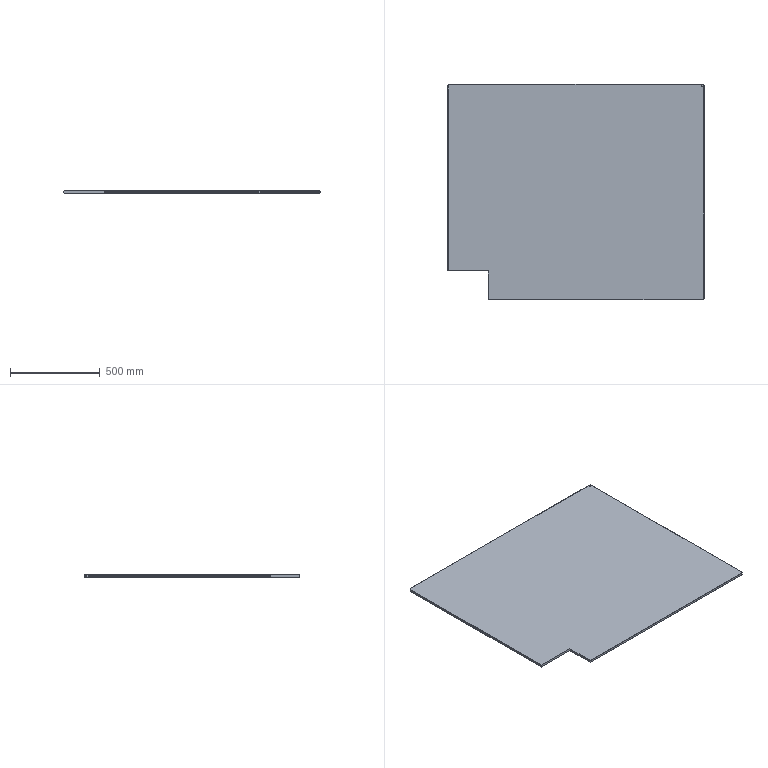Part | STEP file | 1200x1425x13 aluminium plateA-1.STEP | 1 solid | 27 faces | box 1425 x 1200 x 13 mm | volume 21754303 mm3 | plane 16 | cone 6 | cylinder 5 | commonest cylinder face diameters 20 x3 5 x2
STEP:
#1=CARTESIAN_POINT('',(-712.5,-439.4,1.));
#2=VERTEX_POINT('',#1);
#3=CARTESIAN_POINT('',(-711.5,-439.4,0.));
#4=VERTEX_POINT('',#3);
#5=CARTESIAN_POINT('',(-712.5,-439.4,1.));
#6=DIRECTION('',(0.7071,0.,-0.7071));
#7=VECTOR('',#6,1000.);
#8=LINE('',#5,#7);
#9=EDGE_CURVE('',#2,#4,#8,.T.);
#10=ORIENTED_EDGE('',*,*,#9,.T.);
#11=CARTESIAN_POINT('',(-487.5,-439.4,0.));
#12=VERTEX_POINT('',#11);
#13=CARTESIAN_POINT('',(-712.5,-439.4,0.));
#14=DIRECTION('',(1.,0.,0.));
#15=VECTOR('',#14,1000.);
#16=LINE('',#13,#15);
#17=EDGE_CURVE('',#4,#12,#16,.T.);
#18=ORIENTED_EDGE('',*,*,#17,.T.);
#19=CARTESIAN_POINT('',(-487.5,-439.4,13.));
#20=VERTEX_POINT('',#19);
#21=CARTESIAN_POINT('',(-487.5,-439.4,13.));
#22=DIRECTION('',(0.,0.,-1.));
#23=VECTOR('',#22,1000.);
#24=LINE('',#21,#23);
#25=EDGE_CURVE('',#20,#12,#24,.T.);
#26=ORIENTED_EDGE('',*,*,#25,.F.);
#27=CARTESIAN_POINT('',(-711.5,-439.4,13.));
#28=VERTEX_POINT('',#27);
#29=CARTESIAN_POINT('',(-712.5,-439.4,13.));
#30=DIRECTION('',(1.,0.,0.));
#31=VECTOR('',#30,1000.);
#32=LINE('',#29,#31);
#33=EDGE_CURVE('',#28,#20,#32,.T.);
#34=ORIENTED_EDGE('',*,*,#33,.F.);
#35=CARTESIAN_POINT('',(-712.5,-439.4,12.));
#36=VERTEX_POINT('',#35);
#37=CARTESIAN_POINT('',(-711.5,-439.4,13.));
#38=DIRECTION('',(-0.7071,0.,-0.7071));
#39=VECTOR('',#38,1000.);
#40=LINE('',#37,#39);
#41=EDGE_CURVE('',#28,#36,#40,.T.);
#42=ORIENTED_EDGE('',*,*,#41,.T.);
#43=CARTESIAN_POINT('',(-712.5,-439.4,13.));
#44=DIRECTION('',(0.,0.,-1.));
#45=VECTOR('',#44,1000.);
#46=LINE('',#43,#45);
#47=EDGE_CURVE('',#36,#2,#46,.T.);
#48=ORIENTED_EDGE('',*,*,#47,.T.);
#49=EDGE_LOOP('',(#10,#18,#26,#34,#42,#48));
#50=FACE_OUTER_BOUND('',#49,.T.);
#51=CARTESIAN_POINT('',(-712.5,-439.4,13.));
#52=DIRECTION('',(0.,1.,0.));
#53=DIRECTION('',(1.,0.,0.));
#54=AXIS2_PLACEMENT_3D('',#51,#52,#53);
#55=PLANE('',#54);
#56=ADVANCED_FACE('',(#50),#55,.F.);
#57=CARTESIAN_POINT('',(-487.5,-599.,0.));
#58=VERTEX_POINT('',#57);
#59=CARTESIAN_POINT('',(-487.5,-600.,1.));
#60=VERTEX_POINT('',#59);
#61=CARTESIAN_POINT('',(-487.5,-600.,1.));
#62=DIRECTION('',(0.,-0.7071,0.7071));
#63=VECTOR('',#62,1000.);
#64=LINE('',#61,#63);
#65=EDGE_CURVE('',#58,#60,#64,.T.);
#66=ORIENTED_EDGE('',*,*,#65,.T.);
#67=CARTESIAN_POINT('',(-487.5,-600.,12.));
#68=VERTEX_POINT('',#67);
#69=CARTESIAN_POINT('',(-487.5,-600.,13.));
#70=DIRECTION('',(0.,0.,-1.));
#71=VECTOR('',#70,1000.);
#72=LINE('',#69,#71);
#73=EDGE_CURVE('',#68,#60,#72,.T.);
#74=ORIENTED_EDGE('',*,*,#73,.F.);
#75=CARTESIAN_POINT('',(-487.5,-599.,13.));
#76=VERTEX_POINT('',#75);
#77=CARTESIAN_POINT('',(-487.5,-599.,13.));
#78=DIRECTION('',(0.,0.7071,0.7071));
#79=VECTOR('',#78,1000.);
#80=LINE('',#77,#79);
#81=EDGE_CURVE('',#68,#76,#80,.T.);
#82=ORIENTED_EDGE('',*,*,#81,.T.);
#83=CARTESIAN_POINT('',(-487.5,-600.,13.));
#84=DIRECTION('',(0.,-1.,0.));
#85=VECTOR('',#84,1000.);
#86=LINE('',#83,#85);
#87=EDGE_CURVE('',#20,#76,#86,.T.);
#88=ORIENTED_EDGE('',*,*,#87,.F.);
#89=ORIENTED_EDGE('',*,*,#25,.T.);
#90=CARTESIAN_POINT('',(-487.5,-600.,0.));
#91=DIRECTION('',(0.,-1.,0.));
#92=VECTOR('',#91,1000.);
#93=LINE('',#90,#92);
#94=EDGE_CURVE('',#12,#58,#93,.T.);
#95=ORIENTED_EDGE('',*,*,#94,.T.);
#96=EDGE_LOOP('',(#66,#74,#82,#88,#89,#95));
#97=FACE_OUTER_BOUND('',#96,.T.);
#98=CARTESIAN_POINT('',(-487.5,-600.,13.));
#99=DIRECTION('',(1.,0.,0.));
#100=DIRECTION('',(0.,1.,0.));
#101=AXIS2_PLACEMENT_3D('',#98,#99,#100);
#102=PLANE('',#101);
#103=ADVANCED_FACE('',(#97),#102,.F.);
#104=CARTESIAN_POINT('',(702.5,587.5,13.));
#105=VERTEX_POINT('',#104);
#106=CARTESIAN_POINT('',(702.5,587.5,0.));
#107=VERTEX_POINT('',#106);
#108=CARTESIAN_POINT('',(702.5,587.5,0.));
#109=DIRECTION('',(0.,0.,-1.));
#110=VECTOR('',#109,1000.);
#111=LINE('',#108,#110);
#112=EDGE_CURVE('',#105,#107,#111,.T.);
#113=ORIENTED_EDGE('',*,*,#112,.F.);
#114=CARTESIAN_POINT('',(697.5,587.5,13.));
#115=VERTEX_POINT('',#114);
#116=CARTESIAN_POINT('',(700.,587.5,13.));
#117=DIRECTION('',(0.,0.,-1.));
#118=DIRECTION('',(-1.,0.,0.));
#119=AXIS2_PLACEMENT_3D('',#116,#117,#118);
#120=CIRCLE('',#119,2.5);
#121=EDGE_CURVE('',#115,#105,#120,.T.);
#122=ORIENTED_EDGE('',*,*,#121,.F.);
#123=CARTESIAN_POINT('',(697.5,587.5,0.));
#124=VERTEX_POINT('',#123);
#125=CARTESIAN_POINT('',(697.5,587.5,0.));
#126=DIRECTION('',(0.,0.,-1.));
#127=VECTOR('',#126,1000.);
#128=LINE('',#125,#127);
#129=EDGE_CURVE('',#115,#124,#128,.T.);
#130=ORIENTED_EDGE('',*,*,#129,.T.);
#131=CARTESIAN_POINT('',(700.,587.5,0.));
#132=DIRECTION('',(0.,0.,-1.));
#133=DIRECTION('',(-1.,0.,0.));
#134=AXIS2_PLACEMENT_3D('',#131,#132,#133);
#135=CIRCLE('',#134,2.5);
#136=EDGE_CURVE('',#124,#107,#135,.T.);
#137=ORIENTED_EDGE('',*,*,#136,.T.);
#138=EDGE_LOOP('',(#113,#122,#130,#137));
#139=FACE_OUTER_BOUND('',#138,.T.);
#140=CARTESIAN_POINT('',(700.,587.5,0.));
#141=DIRECTION('',(0.,0.,-1.));
#142=DIRECTION('',(-1.,0.,0.));
#143=AXIS2_PLACEMENT_3D('',#140,#141,#142);
#144=CYLINDRICAL_SURFACE('',#143,2.5);
#145=ADVANCED_FACE('',(#139),#144,.F.);
#146=CARTESIAN_POINT('',(-702.5,599.,13.));
#147=VERTEX_POINT('',#146);
#148=CARTESIAN_POINT('',(-702.5,600.,12.));
#149=VERTEX_POINT('',#148);
#150=CARTESIAN_POINT('',(-702.5,599.,13.));
#151=DIRECTION('',(0.,0.7071,-0.7071));
#152=VECTOR('',#151,1000.);
#153=LINE('',#150,#152);
#154=EDGE_CURVE('',#147,#149,#153,.T.);
#155=ORIENTED_EDGE('',*,*,#154,.T.);
#156=CARTESIAN_POINT('',(-712.5,590.,12.));
#157=VERTEX_POINT('',#156);
#158=CARTESIAN_POINT('',(-702.5,590.,12.));
#159=DIRECTION('',(0.,0.,-1.));
#160=DIRECTION('',(1.,0.,0.));
#161=AXIS2_PLACEMENT_3D('',#158,#159,#160);
#162=CIRCLE('',#161,10.);
#163=EDGE_CURVE('',#157,#149,#162,.T.);
#164=ORIENTED_EDGE('',*,*,#163,.F.);
#165=CARTESIAN_POINT('',(-711.5,590.,13.));
#166=VERTEX_POINT('',#165);
#167=CARTESIAN_POINT('',(-712.5,590.,12.));
#168=DIRECTION('',(0.7071,0.,0.7071));
#169=VECTOR('',#168,1000.);
#170=LINE('',#167,#169);
#171=EDGE_CURVE('',#157,#166,#170,.T.);
#172=ORIENTED_EDGE('',*,*,#171,.T.);
#173=CARTESIAN_POINT('',(-702.5,590.,13.));
#174=DIRECTION('',(0.,0.,1.));
#175=DIRECTION('',(1.,0.,0.));
#176=AXIS2_PLACEMENT_3D('',#173,#174,#175);
#177=CIRCLE('',#176,9.);
#178=EDGE_CURVE('',#147,#166,#177,.T.);
#179=ORIENTED_EDGE('',*,*,#178,.F.);
#180=EDGE_LOOP('',(#155,#164,#172,#179));
#181=FACE_OUTER_BOUND('',#180,.T.);
#182=CARTESIAN_POINT('',(-702.5,590.,13.));
#183=DIRECTION('',(0.,0.,-1.));
#184=DIRECTION('',(-1.,0.,0.));
#185=AXIS2_PLACEMENT_3D('',#182,#183,#184);
#186=CONICAL_SURFACE('',#185,9.,0.7854);
#187=ADVANCED_FACE('',(#181),#186,.T.);
#188=ORIENTED_EDGE('',*,*,#41,.F.);
#189=CARTESIAN_POINT('',(-711.5,-590.,13.));
#190=DIRECTION('',(0.,-1.,0.));
#191=VECTOR('',#190,1000.);
#192=LINE('',#189,#191);
#193=EDGE_CURVE('',#166,#28,#192,.T.);
#194=ORIENTED_EDGE('',*,*,#193,.F.);
#195=ORIENTED_EDGE('',*,*,#171,.F.);
#196=CARTESIAN_POINT('',(-712.5,590.,12.));
#197=DIRECTION('',(0.,1.,0.));
#198=VECTOR('',#197,1000.);
#199=LINE('',#196,#198);
#200=EDGE_CURVE('',#36,#157,#199,.T.);
#201=ORIENTED_EDGE('',*,*,#200,.F.);
#202=EDGE_LOOP('',(#188,#194,#195,#201));
#203=FACE_OUTER_BOUND('',#202,.T.);
#204=CARTESIAN_POINT('',(-711.5,0.,13.));
#205=DIRECTION('',(-0.7071,0.,0.7071));
#206=DIRECTION('',(0.,1.,0.));
#207=AXIS2_PLACEMENT_3D('',#204,#205,#206);
#208=PLANE('',#207);
#209=ADVANCED_FACE('',(#203),#208,.T.);
#210=CARTESIAN_POINT('',(702.5,599.,13.));
#211=VERTEX_POINT('',#210);
#212=CARTESIAN_POINT('',(702.5,600.,12.));
#213=VERTEX_POINT('',#212);
#214=CARTESIAN_POINT('',(702.5,599.,13.));
#215=DIRECTION('',(0.,0.7071,-0.7071));
#216=VECTOR('',#215,1000.);
#217=LINE('',#214,#216);
#218=EDGE_CURVE('',#211,#213,#217,.T.);
#219=ORIENTED_EDGE('',*,*,#218,.T.);
#220=CARTESIAN_POINT('',(702.5,600.,12.));
#221=DIRECTION('',(1.,0.,0.));
#222=VECTOR('',#221,1000.);
#223=LINE('',#220,#222);
#224=EDGE_CURVE('',#149,#213,#223,.T.);
#225=ORIENTED_EDGE('',*,*,#224,.F.);
#226=ORIENTED_EDGE('',*,*,#154,.F.);
#227=CARTESIAN_POINT('',(-702.5,599.,13.));
#228=DIRECTION('',(-1.,0.,0.));
#229=VECTOR('',#228,1000.);
#230=LINE('',#227,#229);
#231=EDGE_CURVE('',#211,#147,#230,.T.);
#232=ORIENTED_EDGE('',*,*,#231,.F.);
#233=EDGE_LOOP('',(#219,#225,#226,#232));
#234=FACE_OUTER_BOUND('',#233,.T.);
#235=CARTESIAN_POINT('',(0.,599.,13.));
#236=DIRECTION('',(0.,0.7071,0.7071));
#237=DIRECTION('',(1.,0.,0.));
#238=AXIS2_PLACEMENT_3D('',#235,#236,#237);
#239=PLANE('',#238);
#240=ADVANCED_FACE('',(#234),#239,.T.);
#241=CARTESIAN_POINT('',(711.5,590.,13.));
#242=VERTEX_POINT('',#241);
#243=CARTESIAN_POINT('',(712.5,590.,12.));
#244=VERTEX_POINT('',#243);
#245=CARTESIAN_POINT('',(711.5,590.,13.));
#246=DIRECTION('',(0.7071,0.,-0.7071));
#247=VECTOR('',#246,1000.);
#248=LINE('',#245,#247);
#249=EDGE_CURVE('',#242,#244,#248,.T.);
#250=ORIENTED_EDGE('',*,*,#249,.T.);
#251=CARTESIAN_POINT('',(702.5,590.,12.));
#252=DIRECTION('',(0.,0.,-1.));
#253=DIRECTION('',(1.,0.,0.));
#254=AXIS2_PLACEMENT_3D('',#251,#252,#253);
#255=CIRCLE('',#254,10.);
#256=EDGE_CURVE('',#213,#244,#255,.T.);
#257=ORIENTED_EDGE('',*,*,#256,.F.);
#258=ORIENTED_EDGE('',*,*,#218,.F.);
#259=CARTESIAN_POINT('',(702.5,590.,13.));
#260=DIRECTION('',(0.,0.,1.));
#261=DIRECTION('',(1.,0.,0.));
#262=AXIS2_PLACEMENT_3D('',#259,#260,#261);
#263=CIRCLE('',#262,9.);
#264=EDGE_CURVE('',#242,#211,#263,.T.);
#265=ORIENTED_EDGE('',*,*,#264,.F.);
#266=EDGE_LOOP('',(#250,#257,#258,#265));
#267=FACE_OUTER_BOUND('',#266,.T.);
#268=CARTESIAN_POINT('',(702.5,590.,13.));
#269=DIRECTION('',(0.,0.,-1.));
#270=DIRECTION('',(-1.,0.,0.));
#271=AXIS2_PLACEMENT_3D('',#268,#269,#270);
#272=CONICAL_SURFACE('',#271,9.,0.7854);
#273=ADVANCED_FACE('',(#267),#272,.T.);
#274=ORIENTED_EDGE('',*,*,#81,.F.);
#275=CARTESIAN_POINT('',(702.5,-600.,12.));
#276=VERTEX_POINT('',#275);
#277=CARTESIAN_POINT('',(-702.5,-600.,12.));
#278=DIRECTION('',(-1.,0.,0.));
#279=VECTOR('',#278,1000.);
#280=LINE('',#277,#279);
#281=EDGE_CURVE('',#276,#68,#280,.T.);
#282=ORIENTED_EDGE('',*,*,#281,.F.);
#283=CARTESIAN_POINT('',(702.5,-599.,13.));
#284=VERTEX_POINT('',#283);
#285=CARTESIAN_POINT('',(702.5,-600.,12.));
#286=DIRECTION('',(0.,0.7071,0.7071));
#287=VECTOR('',#286,1000.);
#288=LINE('',#285,#287);
#289=EDGE_CURVE('',#276,#284,#288,.T.);
#290=ORIENTED_EDGE('',*,*,#289,.T.);
#291=CARTESIAN_POINT('',(702.5,-599.,13.));
#292=DIRECTION('',(1.,0.,0.));
#293=VECTOR('',#292,1000.);
#294=LINE('',#291,#293);
#295=EDGE_CURVE('',#76,#284,#294,.T.);
#296=ORIENTED_EDGE('',*,*,#295,.F.);
#297=EDGE_LOOP('',(#274,#282,#290,#296));
#298=FACE_OUTER_BOUND('',#297,.T.);
#299=CARTESIAN_POINT('',(0.,-599.,13.));
#300=DIRECTION('',(0.,-0.7071,0.7071));
#301=DIRECTION('',(-1.,0.,0.));
#302=AXIS2_PLACEMENT_3D('',#299,#300,#301);
#303=PLANE('',#302);
#304=ADVANCED_FACE('',(#298),#303,.T.);
#305=CARTESIAN_POINT('',(711.5,-590.,13.));
#306=VERTEX_POINT('',#305);
#307=CARTESIAN_POINT('',(712.5,-590.,12.));
#308=VERTEX_POINT('',#307);
#309=CARTESIAN_POINT('',(711.5,-590.,13.));
#310=DIRECTION('',(0.7071,0.,-0.7071));
#311=VECTOR('',#310,1000.);
#312=LINE('',#309,#311);
#313=EDGE_CURVE('',#306,#308,#312,.T.);
#314=ORIENTED_EDGE('',*,*,#313,.T.);
#315=CARTESIAN_POINT('',(712.5,-590.,12.));
#316=DIRECTION('',(0.,-1.,0.));
#317=VECTOR('',#316,1000.);
#318=LINE('',#315,#317);
#319=EDGE_CURVE('',#244,#308,#318,.T.);
#320=ORIENTED_EDGE('',*,*,#319,.F.);
#321=ORIENTED_EDGE('',*,*,#249,.F.);
#322=CARTESIAN_POINT('',(711.5,590.,13.));
#323=DIRECTION('',(0.,1.,0.));
#324=VECTOR('',#323,1000.);
#325=LINE('',#322,#324);
#326=EDGE_CURVE('',#306,#242,#325,.T.);
#327=ORIENTED_EDGE('',*,*,#326,.F.);
#328=EDGE_LOOP('',(#314,#320,#321,#327));
#329=FACE_OUTER_BOUND('',#328,.T.);
#330=CARTESIAN_POINT('',(711.5,0.,13.));
#331=DIRECTION('',(0.7071,0.,0.7071));
#332=DIRECTION('',(0.,-1.,0.));
#333=AXIS2_PLACEMENT_3D('',#330,#331,#332);
#334=PLANE('',#333);
#335=ADVANCED_FACE('',(#329),#334,.T.);
#336=ORIENTED_EDGE('',*,*,#289,.F.);
#337=CARTESIAN_POINT('',(702.5,-590.,12.));
#338=DIRECTION('',(0.,0.,-1.));
#339=DIRECTION('',(1.,0.,0.));
#340=AXIS2_PLACEMENT_3D('',#337,#338,#339);
#341=CIRCLE('',#340,10.);
#342=EDGE_CURVE('',#308,#276,#341,.T.);
#343=ORIENTED_EDGE('',*,*,#342,.F.);
#344=ORIENTED_EDGE('',*,*,#313,.F.);
#345=CARTESIAN_POINT('',(702.5,-590.,13.));
#346=DIRECTION('',(0.,0.,1.));
#347=DIRECTION('',(1.,0.,0.));
#348=AXIS2_PLACEMENT_3D('',#345,#346,#347);
#349=CIRCLE('',#348,9.);
#350=EDGE_CURVE('',#284,#306,#349,.T.);
#351=ORIENTED_EDGE('',*,*,#350,.F.);
#352=EDGE_LOOP('',(#336,#343,#344,#351));
#353=FACE_OUTER_BOUND('',#352,.T.);
#354=CARTESIAN_POINT('',(702.5,-590.,13.));
#355=DIRECTION('',(0.,0.,-1.));
#356=DIRECTION('',(-1.,0.,0.));
#357=AXIS2_PLACEMENT_3D('',#354,#355,#356);
#358=CONICAL_SURFACE('',#357,9.,0.7854);
#359=ADVANCED_FACE('',(#353),#358,.T.);
#360=CARTESIAN_POINT('',(711.5,-590.,0.));
#361=VERTEX_POINT('',#360);
#362=CARTESIAN_POINT('',(712.5,-590.,1.));
#363=VERTEX_POINT('',#362);
#364=CARTESIAN_POINT('',(711.5,-590.,0.));
#365=DIRECTION('',(0.7071,0.,0.7071));
#366=VECTOR('',#365,1000.);
#367=LINE('',#364,#366);
#368=EDGE_CURVE('',#361,#363,#367,.T.);
#369=ORIENTED_EDGE('',*,*,#368,.T.);
#370=CARTESIAN_POINT('',(702.5,-600.,1.));
#371=VERTEX_POINT('',#370);
#372=CARTESIAN_POINT('',(702.5,-590.,1.));
#373=DIRECTION('',(0.,0.,1.));
#374=DIRECTION('',(1.,0.,0.));
#375=AXIS2_PLACEMENT_3D('',#372,#373,#374);
#376=CIRCLE('',#375,10.);
#377=EDGE_CURVE('',#371,#363,#376,.T.);
#378=ORIENTED_EDGE('',*,*,#377,.F.);
#379=CARTESIAN_POINT('',(702.5,-599.,0.));
#380=VERTEX_POINT('',#379);
#381=CARTESIAN_POINT('',(702.5,-600.,1.));
#382=DIRECTION('',(0.,0.7071,-0.7071));
#383=VECTOR('',#382,1000.);
#384=LINE('',#381,#383);
#385=EDGE_CURVE('',#371,#380,#384,.T.);
#386=ORIENTED_EDGE('',*,*,#385,.T.);
#387=CARTESIAN_POINT('',(702.5,-590.,0.));
#388=DIRECTION('',(0.,0.,-1.));
#389=DIRECTION('',(1.,0.,0.));
#390=AXIS2_PLACEMENT_3D('',#387,#388,#389);
#391=CIRCLE('',#390,9.);
#392=EDGE_CURVE('',#361,#380,#391,.T.);
#393=ORIENTED_EDGE('',*,*,#392,.F.);
#394=EDGE_LOOP('',(#369,#378,#386,#393));
#395=FACE_OUTER_BOUND('',#394,.T.);
#396=CARTESIAN_POINT('',(702.5,-590.,0.));
#397=DIRECTION('',(0.,0.,1.));
#398=DIRECTION('',(1.,0.,0.));
#399=AXIS2_PLACEMENT_3D('',#396,#397,#398);
#400=CONICAL_SURFACE('',#399,9.,0.7854);
#401=ADVANCED_FACE('',(#395),#400,.T.);
#402=ORIENTED_EDGE('',*,*,#65,.F.);
#403=CARTESIAN_POINT('',(0.,-599.,0.));
#404=DIRECTION('',(-1.,0.,0.));
#405=VECTOR('',#404,1000.);
#406=LINE('',#403,#405);
#407=EDGE_CURVE('',#380,#58,#406,.T.);
#408=ORIENTED_EDGE('',*,*,#407,.F.);
#409=ORIENTED_EDGE('',*,*,#385,.F.);
#410=CARTESIAN_POINT('',(-712.5,-600.,1.));
#411=DIRECTION('',(1.,0.,0.));
#412=VECTOR('',#411,1000.);
#413=LINE('',#410,#412);
#414=EDGE_CURVE('',#60,#371,#413,.T.);
#415=ORIENTED_EDGE('',*,*,#414,.F.);
#416=EDGE_LOOP('',(#402,#408,#409,#415));
#417=FACE_OUTER_BOUND('',#416,.T.);
#418=CARTESIAN_POINT('',(-712.5,-600.,1.));
#419=DIRECTION('',(0.,0.7071,0.7071));
#420=DIRECTION('',(1.,0.,0.));
#421=AXIS2_PLACEMENT_3D('',#418,#419,#420);
#422=PLANE('',#421);
#423=ADVANCED_FACE('',(#417),#422,.F.);
#424=CARTESIAN_POINT('',(711.5,590.,0.));
#425=VERTEX_POINT('',#424);
#426=CARTESIAN_POINT('',(712.5,590.,1.));
#427=VERTEX_POINT('',#426);
#428=CARTESIAN_POINT('',(711.5,590.,0.));
#429=DIRECTION('',(0.7071,0.,0.7071));
#430=VECTOR('',#429,1000.);
#431=LINE('',#428,#430);
#432=EDGE_CURVE('',#425,#427,#431,.T.);
#433=ORIENTED_EDGE('',*,*,#432,.T.);
#434=CARTESIAN_POINT('',(712.5,600.,1.));
#435=DIRECTION('',(0.,1.,0.));
#436=VECTOR('',#435,1000.);
#437=LINE('',#434,#436);
#438=EDGE_CURVE('',#363,#427,#437,.T.);
#439=ORIENTED_EDGE('',*,*,#438,.F.);
#440=ORIENTED_EDGE('',*,*,#368,.F.);
#441=CARTESIAN_POINT('',(711.5,0.,0.));
#442=DIRECTION('',(0.,-1.,0.));
#443=VECTOR('',#442,1000.);
#444=LINE('',#441,#443);
#445=EDGE_CURVE('',#425,#361,#444,.T.);
#446=ORIENTED_EDGE('',*,*,#445,.F.);
#447=EDGE_LOOP('',(#433,#439,#440,#446));
#448=FACE_OUTER_BOUND('',#447,.T.);
#449=CARTESIAN_POINT('',(712.5,600.,1.));
#450=DIRECTION('',(-0.7071,0.,0.7071));
#451=DIRECTION('',(0.,1.,0.));
#452=AXIS2_PLACEMENT_3D('',#449,#450,#451);
#453=PLANE('',#452);
#454=ADVANCED_FACE('',(#448),#453,.F.);
#455=CARTESIAN_POINT('',(702.5,599.,0.));
#456=VERTEX_POINT('',#455);
#457=CARTESIAN_POINT('',(702.5,600.,1.));
#458=VERTEX_POINT('',#457);
#459=CARTESIAN_POINT('',(702.5,599.,0.));
#460=DIRECTION('',(0.,0.7071,0.7071));
#461=VECTOR('',#460,1000.);
#462=LINE('',#459,#461);
#463=EDGE_CURVE('',#456,#458,#462,.T.);
#464=ORIENTED_EDGE('',*,*,#463,.T.);
#465=CARTESIAN_POINT('',(702.5,590.,1.));
#466=DIRECTION('',(0.,0.,1.));
#467=DIRECTION('',(1.,0.,0.));
#468=AXIS2_PLACEMENT_3D('',#465,#466,#467);
#469=CIRCLE('',#468,10.);
#470=EDGE_CURVE('',#427,#458,#469,.T.);
#471=ORIENTED_EDGE('',*,*,#470,.F.);
#472=ORIENTED_EDGE('',*,*,#432,.F.);
#473=CARTESIAN_POINT('',(702.5,590.,0.));
#474=DIRECTION('',(0.,0.,-1.));
#475=DIRECTION('',(1.,0.,0.));
#476=AXIS2_PLACEMENT_3D('',#473,#474,#475);
#477=CIRCLE('',#476,9.);
#478=EDGE_CURVE('',#456,#425,#477,.T.);
#479=ORIENTED_EDGE('',*,*,#478,.F.);
#480=EDGE_LOOP('',(#464,#471,#472,#479));
#481=FACE_OUTER_BOUND('',#480,.T.);
#482=CARTESIAN_POINT('',(702.5,590.,0.));
#483=DIRECTION('',(0.,0.,1.));
#484=DIRECTION('',(1.,0.,0.));
#485=AXIS2_PLACEMENT_3D('',#482,#483,#484);
#486=CONICAL_SURFACE('',#485,9.,0.7854);
#487=ADVANCED_FACE('',(#481),#486,.T.);
#488=ORIENTED_EDGE('',*,*,#9,.F.);
#489=CARTESIAN_POINT('',(-712.5,590.,1.));
#490=VERTEX_POINT('',#489);
#491=CARTESIAN_POINT('',(-712.5,600.,1.));
#492=DIRECTION('',(0.,-1.,0.));
#493=VECTOR('',#492,1000.);
#494=LINE('',#491,#493);
#495=EDGE_CURVE('',#490,#2,#494,.T.);
#496=ORIENTED_EDGE('',*,*,#495,.F.);
#497=CARTESIAN_POINT('',(-711.5,590.,0.));
#498=VERTEX_POINT('',#497);
#499=CARTESIAN_POINT('',(-712.5,590.,1.));
#500=DIRECTION('',(0.7071,0.,-0.7071));
#501=VECTOR('',#500,1000.);
#502=LINE('',#499,#501);
#503=EDGE_CURVE('',#490,#498,#502,.T.);
#504=ORIENTED_EDGE('',*,*,#503,.T.);
#505=CARTESIAN_POINT('',(-711.5,0.,0.));
#506=DIRECTION('',(0.,1.,0.));
#507=VECTOR('',#506,1000.);
#508=LINE('',#505,#507);
#509=EDGE_CURVE('',#4,#498,#508,.T.);
#510=ORIENTED_EDGE('',*,*,#509,.F.);
#511=EDGE_LOOP('',(#488,#496,#504,#510));
#512=FACE_OUTER_BOUND('',#511,.T.);
#513=CARTESIAN_POINT('',(-712.5,600.,1.));
#514=DIRECTION('',(0.7071,0.,0.7071));
#515=DIRECTION('',(0.,-1.,0.));
#516=AXIS2_PLACEMENT_3D('',#513,#514,#515);
#517=PLANE('',#516);
#518=ADVANCED_FACE('',(#512),#517,.F.);
#519=CARTESIAN_POINT('',(-702.5,599.,0.));
#520=VERTEX_POINT('',#519);
#521=CARTESIAN_POINT('',(-702.5,600.,1.));
#522=VERTEX_POINT('',#521);
#523=CARTESIAN_POINT('',(-702.5,599.,0.));
#524=DIRECTION('',(0.,0.7071,0.7071));
#525=VECTOR('',#524,1000.);
#526=LINE('',#523,#525);
#527=EDGE_CURVE('',#520,#522,#526,.T.);
#528=ORIENTED_EDGE('',*,*,#527,.T.);
#529=CARTESIAN_POINT('',(-712.5,600.,1.));
#530=DIRECTION('',(-1.,0.,0.));
#531=VECTOR('',#530,1000.);
#532=LINE('',#529,#531);
#533=EDGE_CURVE('',#458,#522,#532,.T.);
#534=ORIENTED_EDGE('',*,*,#533,.F.);
#535=ORIENTED_EDGE('',*,*,#463,.F.);
#536=CARTESIAN_POINT('',(0.,599.,0.));
#537=DIRECTION('',(1.,0.,0.));
#538=VECTOR('',#537,1000.);
#539=LINE('',#536,#538);
#540=EDGE_CURVE('',#520,#456,#539,.T.);
#541=ORIENTED_EDGE('',*,*,#540,.F.);
#542=EDGE_LOOP('',(#528,#534,#535,#541));
#543=FACE_OUTER_BOUND('',#542,.T.);
#544=CARTESIAN_POINT('',(-712.5,600.,1.));
#545=DIRECTION('',(0.,-0.7071,0.7071));
#546=DIRECTION('',(-1.,0.,0.));
#547=AXIS2_PLACEMENT_3D('',#544,#545,#546);
#548=PLANE('',#547);
#549=ADVANCED_FACE('',(#543),#548,.F.);
#550=ORIENTED_EDGE('',*,*,#503,.F.);
#551=CARTESIAN_POINT('',(-702.5,590.,1.));
#552=DIRECTION('',(0.,0.,1.));
#553=DIRECTION('',(1.,0.,0.));
#554=AXIS2_PLACEMENT_3D('',#551,#552,#553);
#555=CIRCLE('',#554,10.);
#556=EDGE_CURVE('',#522,#490,#555,.T.);
#557=ORIENTED_EDGE('',*,*,#556,.F.);
#558=ORIENTED_EDGE('',*,*,#527,.F.);
#559=CARTESIAN_POINT('',(-702.5,590.,0.));
#560=DIRECTION('',(0.,0.,-1.));
#561=DIRECTION('',(1.,0.,0.));
#562=AXIS2_PLACEMENT_3D('',#559,#560,#561);
#563=CIRCLE('',#562,9.);
#564=EDGE_CURVE('',#498,#520,#563,.T.);
#565=ORIENTED_EDGE('',*,*,#564,.F.);
#566=EDGE_LOOP('',(#550,#557,#558,#565));
#567=FACE_OUTER_BOUND('',#566,.T.);
#568=CARTESIAN_POINT('',(-702.5,590.,0.));
#569=DIRECTION('',(0.,0.,1.));
#570=DIRECTION('',(1.,0.,0.));
#571=AXIS2_PLACEMENT_3D('',#568,#569,#570);
#572=CONICAL_SURFACE('',#571,9.,0.7854);
#573=ADVANCED_FACE('',(#567),#572,.T.);
#574=CARTESIAN_POINT('',(-702.5,600.,13.));
#575=DIRECTION('',(0.,0.,1.));
#576=VECTOR('',#575,1000.);
#577=LINE('',#574,#576);
#578=EDGE_CURVE('',#522,#149,#577,.T.);
#579=ORIENTED_EDGE('',*,*,#578,.F.);
#580=ORIENTED_EDGE('',*,*,#556,.T.);
#581=CARTESIAN_POINT('',(-712.5,590.,13.));
#582=DIRECTION('',(0.,0.,-1.));
#583=VECTOR('',#582,1000.);
#584=LINE('',#581,#583);
#585=EDGE_CURVE('',#157,#490,#584,.T.);
#586=ORIENTED_EDGE('',*,*,#585,.F.);
#587=ORIENTED_EDGE('',*,*,#163,.T.);
#588=EDGE_LOOP('',(#579,#580,#586,#587));
#589=FACE_OUTER_BOUND('',#588,.T.);
#590=CARTESIAN_POINT('',(-702.5,590.,13.));
#591=DIRECTION('',(0.,0.,-1.));
#592=DIRECTION('',(-1.,0.,0.));
#593=AXIS2_PLACEMENT_3D('',#590,#591,#592);
#594=CYLINDRICAL_SURFACE('',#593,10.);
#595=ADVANCED_FACE('',(#589),#594,.T.);
#596=CARTESIAN_POINT('',(712.5,590.,13.));
#597=DIRECTION('',(0.,0.,1.));
#598=VECTOR('',#597,1000.);
#599=LINE('',#596,#598);
#600=EDGE_CURVE('',#427,#244,#599,.T.);
#601=ORIENTED_EDGE('',*,*,#600,.F.);
#602=ORIENTED_EDGE('',*,*,#470,.T.);
#603=CARTESIAN_POINT('',(702.5,600.,13.));
#604=DIRECTION('',(0.,0.,-1.));
#605=VECTOR('',#604,1000.);
#606=LINE('',#603,#605);
#607=EDGE_CURVE('',#213,#458,#606,.T.);
#608=ORIENTED_EDGE('',*,*,#607,.F.);
#609=ORIENTED_EDGE('',*,*,#256,.T.);
#610=EDGE_LOOP('',(#601,#602,#608,#609));
#611=FACE_OUTER_BOUND('',#610,.T.);
#612=CARTESIAN_POINT('',(702.5,590.,13.));
#613=DIRECTION('',(0.,0.,-1.));
#614=DIRECTION('',(-1.,0.,0.));
#615=AXIS2_PLACEMENT_3D('',#612,#613,#614);
#616=CYLINDRICAL_SURFACE('',#615,10.);
#617=ADVANCED_FACE('',(#611),#616,.T.);
#618=CARTESIAN_POINT('',(702.5,-600.,13.));
#619=DIRECTION('',(0.,0.,1.));
#620=VECTOR('',#619,1000.);
#621=LINE('',#618,#620);
#622=EDGE_CURVE('',#371,#276,#621,.T.);
#623=ORIENTED_EDGE('',*,*,#622,.F.);
#624=ORIENTED_EDGE('',*,*,#377,.T.);
#625=CARTESIAN_POINT('',(712.5,-590.,13.));
#626=DIRECTION('',(0.,0.,-1.));
#627=VECTOR('',#626,1000.);
#628=LINE('',#625,#627);
#629=EDGE_CURVE('',#308,#363,#628,.T.);
#630=ORIENTED_EDGE('',*,*,#629,.F.);
#631=ORIENTED_EDGE('',*,*,#342,.T.);
#632=EDGE_LOOP('',(#623,#624,#630,#631));
#633=FACE_OUTER_BOUND('',#632,.T.);
#634=CARTESIAN_POINT('',(702.5,-590.,13.));
#635=DIRECTION('',(0.,0.,-1.));
#636=DIRECTION('',(-1.,0.,0.));
#637=AXIS2_PLACEMENT_3D('',#634,#635,#636);
#638=CYLINDRICAL_SURFACE('',#637,10.);
#639=ADVANCED_FACE('',(#633),#638,.T.);
#640=ORIENTED_EDGE('',*,*,#136,.F.);
#641=CARTESIAN_POINT('',(700.,587.5,0.));
#642=DIRECTION('',(0.,0.,-1.));
#643=DIRECTION('',(-1.,0.,0.));
#644=AXIS2_PLACEMENT_3D('',#641,#642,#643);
#645=CIRCLE('',#644,2.5);
#646=EDGE_CURVE('',#107,#124,#645,.T.);
#647=ORIENTED_EDGE('',*,*,#646,.F.);
#648=EDGE_LOOP('',(#640,#647));
#649=FACE_BOUND('',#648,.T.);
#650=ORIENTED_EDGE('',*,*,#407,.T.);
#651=ORIENTED_EDGE('',*,*,#94,.F.);
#652=ORIENTED_EDGE('',*,*,#17,.F.);
#653=ORIENTED_EDGE('',*,*,#509,.T.);
#654=ORIENTED_EDGE('',*,*,#564,.T.);
#655=ORIENTED_EDGE('',*,*,#540,.T.);
#656=ORIENTED_EDGE('',*,*,#478,.T.);
#657=ORIENTED_EDGE('',*,*,#445,.T.);
#658=ORIENTED_EDGE('',*,*,#392,.T.);
#659=EDGE_LOOP('',(#650,#651,#652,#653,#654,#655,#656,#657,#658));
#660=FACE_OUTER_BOUND('',#659,.T.);
#661=CARTESIAN_POINT('',(0.,0.,0.));
#662=DIRECTION('',(0.,0.,1.));
#663=DIRECTION('',(1.,0.,0.));
#664=AXIS2_PLACEMENT_3D('',#661,#662,#663);
#665=PLANE('',#664);
#666=ADVANCED_FACE('',(#649,#660),#665,.F.);
#667=ORIENTED_EDGE('',*,*,#121,.T.);
#668=CARTESIAN_POINT('',(700.,587.5,13.));
#669=DIRECTION('',(0.,0.,-1.));
#670=DIRECTION('',(-1.,0.,0.));
#671=AXIS2_PLACEMENT_3D('',#668,#669,#670);
#672=CIRCLE('',#671,2.5);
#673=EDGE_CURVE('',#105,#115,#672,.T.);
#674=ORIENTED_EDGE('',*,*,#673,.T.);
#675=EDGE_LOOP('',(#667,#674));
#676=FACE_BOUND('',#675,.T.);
#677=ORIENTED_EDGE('',*,*,#87,.T.);
#678=ORIENTED_EDGE('',*,*,#295,.T.);
#679=ORIENTED_EDGE('',*,*,#350,.T.);
#680=ORIENTED_EDGE('',*,*,#326,.T.);
#681=ORIENTED_EDGE('',*,*,#264,.T.);
#682=ORIENTED_EDGE('',*,*,#231,.T.);
#683=ORIENTED_EDGE('',*,*,#178,.T.);
#684=ORIENTED_EDGE('',*,*,#193,.T.);
#685=ORIENTED_EDGE('',*,*,#33,.T.);
#686=EDGE_LOOP('',(#677,#678,#679,#680,#681,#682,#683,#684,#685));
#687=FACE_OUTER_BOUND('',#686,.T.);
#688=CARTESIAN_POINT('',(0.,0.,13.));
#689=DIRECTION('',(0.,0.,1.));
#690=DIRECTION('',(1.,0.,0.));
#691=AXIS2_PLACEMENT_3D('',#688,#689,#690);
#692=PLANE('',#691);
#693=ADVANCED_FACE('',(#676,#687),#692,.T.);
#694=ORIENTED_EDGE('',*,*,#281,.T.);
#695=ORIENTED_EDGE('',*,*,#73,.T.);
#696=ORIENTED_EDGE('',*,*,#414,.T.);
#697=ORIENTED_EDGE('',*,*,#622,.T.);
#698=EDGE_LOOP('',(#694,#695,#696,#697));
#699=FACE_OUTER_BOUND('',#698,.T.);
#700=CARTESIAN_POINT('',(-712.5,-600.,13.));
#701=DIRECTION('',(0.,1.,0.));
#702=DIRECTION('',(1.,0.,0.));
#703=AXIS2_PLACEMENT_3D('',#700,#701,#702);
#704=PLANE('',#703);
#705=ADVANCED_FACE('',(#699),#704,.F.);
#706=ORIENTED_EDGE('',*,*,#495,.T.);
#707=ORIENTED_EDGE('',*,*,#47,.F.);
#708=ORIENTED_EDGE('',*,*,#200,.T.);
#709=ORIENTED_EDGE('',*,*,#585,.T.);
#710=EDGE_LOOP('',(#706,#707,#708,#709));
#711=FACE_OUTER_BOUND('',#710,.T.);
#712=CARTESIAN_POINT('',(-712.5,600.,13.));
#713=DIRECTION('',(1.,0.,0.));
#714=DIRECTION('',(0.,1.,0.));
#715=AXIS2_PLACEMENT_3D('',#712,#713,#714);
#716=PLANE('',#715);
#717=ADVANCED_FACE('',(#711),#716,.F.);
#718=ORIENTED_EDGE('',*,*,#607,.T.);
#719=ORIENTED_EDGE('',*,*,#533,.T.);
#720=ORIENTED_EDGE('',*,*,#578,.T.);
#721=ORIENTED_EDGE('',*,*,#224,.T.);
#722=EDGE_LOOP('',(#718,#719,#720,#721));
#723=FACE_OUTER_BOUND('',#722,.T.);
#724=CARTESIAN_POINT('',(-712.5,600.,13.));
#725=DIRECTION('',(0.,-1.,0.));
#726=DIRECTION('',(0.,0.,-1.));
#727=AXIS2_PLACEMENT_3D('',#724,#725,#726);
#728=PLANE('',#727);
#729=ADVANCED_FACE('',(#723),#728,.F.);
#730=ORIENTED_EDGE('',*,*,#629,.T.);
#731=ORIENTED_EDGE('',*,*,#438,.T.);
#732=ORIENTED_EDGE('',*,*,#600,.T.);
#733=ORIENTED_EDGE('',*,*,#319,.T.);
#734=EDGE_LOOP('',(#730,#731,#732,#733));
#735=FACE_OUTER_BOUND('',#734,.T.);
#736=CARTESIAN_POINT('',(712.5,600.,13.));
#737=DIRECTION('',(-1.,0.,0.));
#738=DIRECTION('',(0.,1.,0.));
#739=AXIS2_PLACEMENT_3D('',#736,#737,#738);
#740=PLANE('',#739);
#741=ADVANCED_FACE('',(#735),#740,.F.);
#742=ORIENTED_EDGE('',*,*,#673,.F.);
#743=ORIENTED_EDGE('',*,*,#112,.T.);
#744=ORIENTED_EDGE('',*,*,#646,.T.);
#745=ORIENTED_EDGE('',*,*,#129,.F.);
#746=EDGE_LOOP('',(#742,#743,#744,#745));
#747=FACE_OUTER_BOUND('',#746,.T.);
#748=CARTESIAN_POINT('',(700.,587.5,0.));
#749=DIRECTION('',(0.,0.,-1.));
#750=DIRECTION('',(-1.,0.,0.));
#751=AXIS2_PLACEMENT_3D('',#748,#749,#750);
#752=CYLINDRICAL_SURFACE('',#751,2.5);
#753=ADVANCED_FACE('',(#747),#752,.F.);
#754=CLOSED_SHELL('',(#56,#103,#145,#187,#209,#240,#273,#304,#335,#359,#401,#423,#454,#487,#518,#549,#573,#595,#617,#639,#666,#693,#705,#717,#729,#741,#753));
#755=MANIFOLD_SOLID_BREP('',#754);
#756=CARTESIAN_POINT('',(0.,0.,0.));
#757=DIRECTION('',(0.,0.,1.));
#758=DIRECTION('',(1.,0.,0.));
#759=AXIS2_PLACEMENT_3D('',#756,#757,#758);
#760=(LENGTH_UNIT()NAMED_UNIT(*)SI_UNIT(.MILLI.,.METRE.));
#761=UNCERTAINTY_MEASURE_WITH_UNIT(LENGTH_MEASURE(0.00001),#760,'','');
#762=(NAMED_UNIT(*)PLANE_ANGLE_UNIT()SI_UNIT($,.RADIAN.));
#763=(NAMED_UNIT(*)SI_UNIT($,.STERADIAN.)SOLID_ANGLE_UNIT());
#764=(GEOMETRIC_REPRESENTATION_CONTEXT(3)GLOBAL_UNCERTAINTY_ASSIGNED_CONTEXT((#761))GLOBAL_UNIT_ASSIGNED_CONTEXT((#760,#762,#763))REPRESENTATION_CONTEXT('',''));
#765=ADVANCED_BREP_SHAPE_REPRESENTATION('',(#755,#759),#764);